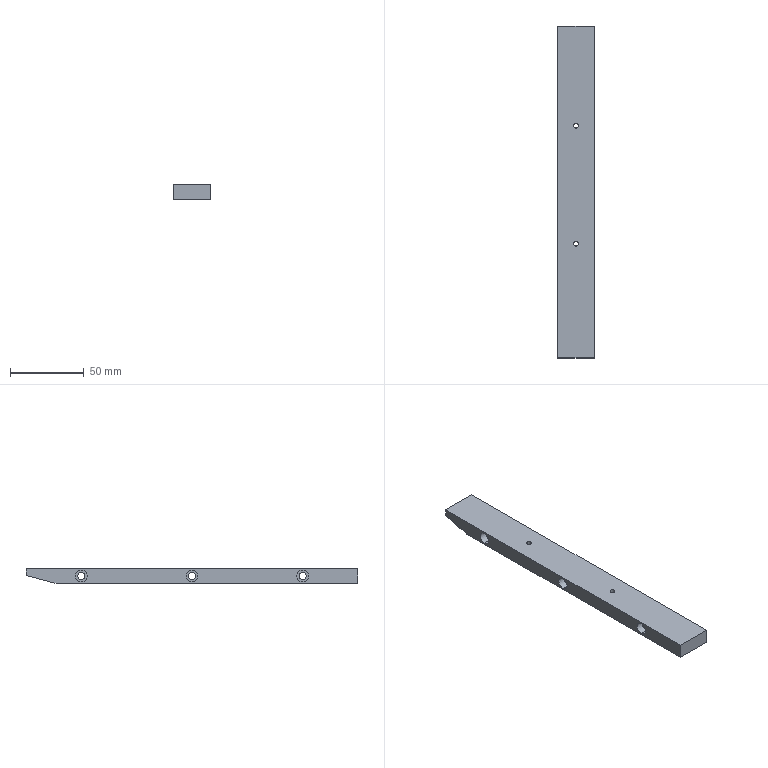Part | SolidWorks | features Chamfer 2, HoleWzd 2, Extrusion 1, Fillet 1 | 1 solid | 27 faces | box 25 x 225 x 10 mm | volume 52898 mm3 | cylinder 17 | plane 10 | commonest cylinder face diameters 4.8 x6 8 x6 3.3 x4 20 x1
STEP:
#1=CARTESIAN_POINT('',(-1.65,45.,-5.));
#2=VERTEX_POINT('',#1);
#3=CARTESIAN_POINT('',(1.65,45.,-5.));
#4=VERTEX_POINT('',#3);
#5=CARTESIAN_POINT('',(0.,45.,-5.));
#6=DIRECTION('',(0.,0.,1.));
#7=DIRECTION('',(1.,0.,0.));
#8=AXIS2_PLACEMENT_3D('',#5,#6,#7);
#9=CIRCLE('',#8,1.65);
#10=EDGE_CURVE('',#2,#4,#9,.T.);
#11=ORIENTED_EDGE('',*,*,#10,.F.);
#12=CARTESIAN_POINT('',(-1.65,45.,5.));
#13=VERTEX_POINT('',#12);
#14=CARTESIAN_POINT('',(-1.65,45.,5.));
#15=DIRECTION('',(0.,0.,1.));
#16=VECTOR('',#15,1000.);
#17=LINE('',#14,#16);
#18=EDGE_CURVE('',#2,#13,#17,.T.);
#19=ORIENTED_EDGE('',*,*,#18,.T.);
#20=CARTESIAN_POINT('',(1.65,45.,5.));
#21=VERTEX_POINT('',#20);
#22=CARTESIAN_POINT('',(0.,45.,5.));
#23=DIRECTION('',(0.,0.,1.));
#24=DIRECTION('',(1.,0.,0.));
#25=AXIS2_PLACEMENT_3D('',#22,#23,#24);
#26=CIRCLE('',#25,1.65);
#27=EDGE_CURVE('',#13,#21,#26,.T.);
#28=ORIENTED_EDGE('',*,*,#27,.T.);
#29=CARTESIAN_POINT('',(1.65,45.,5.));
#30=DIRECTION('',(0.,0.,1.));
#31=VECTOR('',#30,1000.);
#32=LINE('',#29,#31);
#33=EDGE_CURVE('',#4,#21,#32,.T.);
#34=ORIENTED_EDGE('',*,*,#33,.F.);
#35=EDGE_LOOP('',(#11,#19,#28,#34));
#36=FACE_OUTER_BOUND('',#35,.T.);
#37=CARTESIAN_POINT('',(0.,45.,5.));
#38=DIRECTION('',(0.,0.,1.));
#39=DIRECTION('',(1.,0.,0.));
#40=AXIS2_PLACEMENT_3D('',#37,#38,#39);
#41=CYLINDRICAL_SURFACE('',#40,1.65);
#42=ADVANCED_FACE('',(#36),#41,.F.);
#43=CARTESIAN_POINT('',(-1.65,-35.,-5.));
#44=VERTEX_POINT('',#43);
#45=CARTESIAN_POINT('',(1.65,-35.,-5.));
#46=VERTEX_POINT('',#45);
#47=CARTESIAN_POINT('',(0.,-35.,-5.));
#48=DIRECTION('',(0.,0.,1.));
#49=DIRECTION('',(1.,0.,0.));
#50=AXIS2_PLACEMENT_3D('',#47,#48,#49);
#51=CIRCLE('',#50,1.65);
#52=EDGE_CURVE('',#44,#46,#51,.T.);
#53=ORIENTED_EDGE('',*,*,#52,.F.);
#54=CARTESIAN_POINT('',(-1.65,-35.,5.));
#55=VERTEX_POINT('',#54);
#56=CARTESIAN_POINT('',(-1.65,-35.,5.));
#57=DIRECTION('',(0.,0.,1.));
#58=VECTOR('',#57,1000.);
#59=LINE('',#56,#58);
#60=EDGE_CURVE('',#44,#55,#59,.T.);
#61=ORIENTED_EDGE('',*,*,#60,.T.);
#62=CARTESIAN_POINT('',(1.65,-35.,5.));
#63=VERTEX_POINT('',#62);
#64=CARTESIAN_POINT('',(0.,-35.,5.));
#65=DIRECTION('',(0.,0.,1.));
#66=DIRECTION('',(1.,0.,0.));
#67=AXIS2_PLACEMENT_3D('',#64,#65,#66);
#68=CIRCLE('',#67,1.65);
#69=EDGE_CURVE('',#55,#63,#68,.T.);
#70=ORIENTED_EDGE('',*,*,#69,.T.);
#71=CARTESIAN_POINT('',(1.65,-35.,5.));
#72=DIRECTION('',(0.,0.,1.));
#73=VECTOR('',#72,1000.);
#74=LINE('',#71,#73);
#75=EDGE_CURVE('',#46,#63,#74,.T.);
#76=ORIENTED_EDGE('',*,*,#75,.F.);
#77=EDGE_LOOP('',(#53,#61,#70,#76));
#78=FACE_OUTER_BOUND('',#77,.T.);
#79=CARTESIAN_POINT('',(0.,-35.,5.));
#80=DIRECTION('',(0.,0.,1.));
#81=DIRECTION('',(1.,0.,0.));
#82=AXIS2_PLACEMENT_3D('',#79,#80,#81);
#83=CYLINDRICAL_SURFACE('',#82,1.65);
#84=ADVANCED_FACE('',(#78),#83,.F.);
#85=CARTESIAN_POINT('',(-7.5,75.,-4.));
#86=VERTEX_POINT('',#85);
#87=CARTESIAN_POINT('',(-7.5,75.,4.));
#88=VERTEX_POINT('',#87);
#89=CARTESIAN_POINT('',(-7.5,75.,0.));
#90=DIRECTION('',(-1.,0.,0.));
#91=DIRECTION('',(0.,0.,1.));
#92=AXIS2_PLACEMENT_3D('',#89,#90,#91);
#93=CIRCLE('',#92,4.);
#94=EDGE_CURVE('',#86,#88,#93,.T.);
#95=ORIENTED_EDGE('',*,*,#94,.F.);
#96=CARTESIAN_POINT('',(-12.5,75.,-4.));
#97=VERTEX_POINT('',#96);
#98=CARTESIAN_POINT('',(-12.5,75.,-4.));
#99=DIRECTION('',(-1.,0.,0.));
#100=VECTOR('',#99,1000.);
#101=LINE('',#98,#100);
#102=EDGE_CURVE('',#86,#97,#101,.T.);
#103=ORIENTED_EDGE('',*,*,#102,.T.);
#104=CARTESIAN_POINT('',(-12.5,75.,4.));
#105=VERTEX_POINT('',#104);
#106=CARTESIAN_POINT('',(-12.5,75.,0.));
#107=DIRECTION('',(-1.,0.,0.));
#108=DIRECTION('',(0.,0.,1.));
#109=AXIS2_PLACEMENT_3D('',#106,#107,#108);
#110=CIRCLE('',#109,4.);
#111=EDGE_CURVE('',#97,#105,#110,.T.);
#112=ORIENTED_EDGE('',*,*,#111,.T.);
#113=CARTESIAN_POINT('',(-12.5,75.,4.));
#114=DIRECTION('',(-1.,0.,0.));
#115=VECTOR('',#114,1000.);
#116=LINE('',#113,#115);
#117=EDGE_CURVE('',#88,#105,#116,.T.);
#118=ORIENTED_EDGE('',*,*,#117,.F.);
#119=EDGE_LOOP('',(#95,#103,#112,#118));
#120=FACE_OUTER_BOUND('',#119,.T.);
#121=CARTESIAN_POINT('',(-12.5,75.,0.));
#122=DIRECTION('',(-1.,0.,0.));
#123=DIRECTION('',(0.,0.,1.));
#124=AXIS2_PLACEMENT_3D('',#121,#122,#123);
#125=CYLINDRICAL_SURFACE('',#124,4.);
#126=ADVANCED_FACE('',(#120),#125,.F.);
#127=CARTESIAN_POINT('',(12.5,75.,-2.4));
#128=VERTEX_POINT('',#127);
#129=CARTESIAN_POINT('',(12.5,75.,2.4));
#130=VERTEX_POINT('',#129);
#131=CARTESIAN_POINT('',(12.5,75.,0.));
#132=DIRECTION('',(-1.,0.,0.));
#133=DIRECTION('',(0.,0.,1.));
#134=AXIS2_PLACEMENT_3D('',#131,#132,#133);
#135=CIRCLE('',#134,2.4);
#136=EDGE_CURVE('',#128,#130,#135,.T.);
#137=ORIENTED_EDGE('',*,*,#136,.F.);
#138=CARTESIAN_POINT('',(-7.5,75.,-2.4));
#139=VERTEX_POINT('',#138);
#140=CARTESIAN_POINT('',(-12.5,75.,-2.4));
#141=DIRECTION('',(-1.,0.,0.));
#142=VECTOR('',#141,1000.);
#143=LINE('',#140,#142);
#144=EDGE_CURVE('',#128,#139,#143,.T.);
#145=ORIENTED_EDGE('',*,*,#144,.T.);
#146=CARTESIAN_POINT('',(-7.5,75.,2.4));
#147=VERTEX_POINT('',#146);
#148=CARTESIAN_POINT('',(-7.5,75.,0.));
#149=DIRECTION('',(-1.,0.,0.));
#150=DIRECTION('',(0.,0.,1.));
#151=AXIS2_PLACEMENT_3D('',#148,#149,#150);
#152=CIRCLE('',#151,2.4);
#153=EDGE_CURVE('',#139,#147,#152,.T.);
#154=ORIENTED_EDGE('',*,*,#153,.T.);
#155=CARTESIAN_POINT('',(-12.5,75.,2.4));
#156=DIRECTION('',(-1.,0.,0.));
#157=VECTOR('',#156,1000.);
#158=LINE('',#155,#157);
#159=EDGE_CURVE('',#130,#147,#158,.T.);
#160=ORIENTED_EDGE('',*,*,#159,.F.);
#161=EDGE_LOOP('',(#137,#145,#154,#160));
#162=FACE_OUTER_BOUND('',#161,.T.);
#163=CARTESIAN_POINT('',(-12.5,75.,0.));
#164=DIRECTION('',(-1.,0.,0.));
#165=DIRECTION('',(0.,0.,1.));
#166=AXIS2_PLACEMENT_3D('',#163,#164,#165);
#167=CYLINDRICAL_SURFACE('',#166,2.4);
#168=ADVANCED_FACE('',(#162),#167,.F.);
#169=CARTESIAN_POINT('',(-7.5,0.,-4.));
#170=VERTEX_POINT('',#169);
#171=CARTESIAN_POINT('',(-7.5,0.,4.));
#172=VERTEX_POINT('',#171);
#173=CARTESIAN_POINT('',(-7.5,0.,0.));
#174=DIRECTION('',(-1.,0.,0.));
#175=DIRECTION('',(0.,0.,1.));
#176=AXIS2_PLACEMENT_3D('',#173,#174,#175);
#177=CIRCLE('',#176,4.);
#178=EDGE_CURVE('',#170,#172,#177,.T.);
#179=ORIENTED_EDGE('',*,*,#178,.F.);
#180=CARTESIAN_POINT('',(-12.5,0.,-4.));
#181=VERTEX_POINT('',#180);
#182=CARTESIAN_POINT('',(-12.5,0.,-4.));
#183=DIRECTION('',(-1.,0.,0.));
#184=VECTOR('',#183,1000.);
#185=LINE('',#182,#184);
#186=EDGE_CURVE('',#170,#181,#185,.T.);
#187=ORIENTED_EDGE('',*,*,#186,.T.);
#188=CARTESIAN_POINT('',(-12.5,0.,4.));
#189=VERTEX_POINT('',#188);
#190=CARTESIAN_POINT('',(-12.5,0.,0.));
#191=DIRECTION('',(-1.,0.,0.));
#192=DIRECTION('',(0.,0.,1.));
#193=AXIS2_PLACEMENT_3D('',#190,#191,#192);
#194=CIRCLE('',#193,4.);
#195=EDGE_CURVE('',#181,#189,#194,.T.);
#196=ORIENTED_EDGE('',*,*,#195,.T.);
#197=CARTESIAN_POINT('',(-12.5,0.,4.));
#198=DIRECTION('',(-1.,0.,0.));
#199=VECTOR('',#198,1000.);
#200=LINE('',#197,#199);
#201=EDGE_CURVE('',#172,#189,#200,.T.);
#202=ORIENTED_EDGE('',*,*,#201,.F.);
#203=EDGE_LOOP('',(#179,#187,#196,#202));
#204=FACE_OUTER_BOUND('',#203,.T.);
#205=CARTESIAN_POINT('',(-12.5,0.,0.));
#206=DIRECTION('',(-1.,0.,0.));
#207=DIRECTION('',(0.,0.,1.));
#208=AXIS2_PLACEMENT_3D('',#205,#206,#207);
#209=CYLINDRICAL_SURFACE('',#208,4.);
#210=ADVANCED_FACE('',(#204),#209,.F.);
#211=CARTESIAN_POINT('',(12.5,0.,-2.4));
#212=VERTEX_POINT('',#211);
#213=CARTESIAN_POINT('',(12.5,0.,2.4));
#214=VERTEX_POINT('',#213);
#215=CARTESIAN_POINT('',(12.5,0.,0.));
#216=DIRECTION('',(-1.,0.,0.));
#217=DIRECTION('',(0.,0.,1.));
#218=AXIS2_PLACEMENT_3D('',#215,#216,#217);
#219=CIRCLE('',#218,2.4);
#220=EDGE_CURVE('',#212,#214,#219,.T.);
#221=ORIENTED_EDGE('',*,*,#220,.F.);
#222=CARTESIAN_POINT('',(-7.5,0.,-2.4));
#223=VERTEX_POINT('',#222);
#224=CARTESIAN_POINT('',(-12.5,0.,-2.4));
#225=DIRECTION('',(-1.,0.,0.));
#226=VECTOR('',#225,1000.);
#227=LINE('',#224,#226);
#228=EDGE_CURVE('',#212,#223,#227,.T.);
#229=ORIENTED_EDGE('',*,*,#228,.T.);
#230=CARTESIAN_POINT('',(-7.5,0.,2.4));
#231=VERTEX_POINT('',#230);
#232=CARTESIAN_POINT('',(-7.5,0.,0.));
#233=DIRECTION('',(-1.,0.,0.));
#234=DIRECTION('',(0.,0.,1.));
#235=AXIS2_PLACEMENT_3D('',#232,#233,#234);
#236=CIRCLE('',#235,2.4);
#237=EDGE_CURVE('',#223,#231,#236,.T.);
#238=ORIENTED_EDGE('',*,*,#237,.T.);
#239=CARTESIAN_POINT('',(-12.5,0.,2.4));
#240=DIRECTION('',(-1.,0.,0.));
#241=VECTOR('',#240,1000.);
#242=LINE('',#239,#241);
#243=EDGE_CURVE('',#214,#231,#242,.T.);
#244=ORIENTED_EDGE('',*,*,#243,.F.);
#245=EDGE_LOOP('',(#221,#229,#238,#244));
#246=FACE_OUTER_BOUND('',#245,.T.);
#247=CARTESIAN_POINT('',(-12.5,0.,0.));
#248=DIRECTION('',(-1.,0.,0.));
#249=DIRECTION('',(0.,0.,1.));
#250=AXIS2_PLACEMENT_3D('',#247,#248,#249);
#251=CYLINDRICAL_SURFACE('',#250,2.4);
#252=ADVANCED_FACE('',(#246),#251,.F.);
#253=CARTESIAN_POINT('',(-7.5,-75.,-4.));
#254=VERTEX_POINT('',#253);
#255=CARTESIAN_POINT('',(-7.5,-75.,4.));
#256=VERTEX_POINT('',#255);
#257=CARTESIAN_POINT('',(-7.5,-75.,0.));
#258=DIRECTION('',(-1.,0.,0.));
#259=DIRECTION('',(0.,0.,1.));
#260=AXIS2_PLACEMENT_3D('',#257,#258,#259);
#261=CIRCLE('',#260,4.);
#262=EDGE_CURVE('',#254,#256,#261,.T.);
#263=ORIENTED_EDGE('',*,*,#262,.F.);
#264=CARTESIAN_POINT('',(-12.5,-75.,-4.));
#265=VERTEX_POINT('',#264);
#266=CARTESIAN_POINT('',(-12.5,-75.,-4.));
#267=DIRECTION('',(-1.,0.,0.));
#268=VECTOR('',#267,1000.);
#269=LINE('',#266,#268);
#270=EDGE_CURVE('',#254,#265,#269,.T.);
#271=ORIENTED_EDGE('',*,*,#270,.T.);
#272=CARTESIAN_POINT('',(-12.5,-75.,4.));
#273=VERTEX_POINT('',#272);
#274=CARTESIAN_POINT('',(-12.5,-75.,0.));
#275=DIRECTION('',(-1.,0.,0.));
#276=DIRECTION('',(0.,0.,1.));
#277=AXIS2_PLACEMENT_3D('',#274,#275,#276);
#278=CIRCLE('',#277,4.);
#279=EDGE_CURVE('',#265,#273,#278,.T.);
#280=ORIENTED_EDGE('',*,*,#279,.T.);
#281=CARTESIAN_POINT('',(-12.5,-75.,4.));
#282=DIRECTION('',(-1.,0.,0.));
#283=VECTOR('',#282,1000.);
#284=LINE('',#281,#283);
#285=EDGE_CURVE('',#256,#273,#284,.T.);
#286=ORIENTED_EDGE('',*,*,#285,.F.);
#287=EDGE_LOOP('',(#263,#271,#280,#286));
#288=FACE_OUTER_BOUND('',#287,.T.);
#289=CARTESIAN_POINT('',(-12.5,-75.,0.));
#290=DIRECTION('',(-1.,0.,0.));
#291=DIRECTION('',(0.,0.,1.));
#292=AXIS2_PLACEMENT_3D('',#289,#290,#291);
#293=CYLINDRICAL_SURFACE('',#292,4.);
#294=ADVANCED_FACE('',(#288),#293,.F.);
#295=CARTESIAN_POINT('',(12.5,-75.,-2.4));
#296=VERTEX_POINT('',#295);
#297=CARTESIAN_POINT('',(12.5,-75.,2.4));
#298=VERTEX_POINT('',#297);
#299=CARTESIAN_POINT('',(12.5,-75.,0.));
#300=DIRECTION('',(-1.,0.,0.));
#301=DIRECTION('',(0.,0.,1.));
#302=AXIS2_PLACEMENT_3D('',#299,#300,#301);
#303=CIRCLE('',#302,2.4);
#304=EDGE_CURVE('',#296,#298,#303,.T.);
#305=ORIENTED_EDGE('',*,*,#304,.F.);
#306=CARTESIAN_POINT('',(-7.5,-75.,-2.4));
#307=VERTEX_POINT('',#306);
#308=CARTESIAN_POINT('',(-12.5,-75.,-2.4));
#309=DIRECTION('',(-1.,0.,0.));
#310=VECTOR('',#309,1000.);
#311=LINE('',#308,#310);
#312=EDGE_CURVE('',#296,#307,#311,.T.);
#313=ORIENTED_EDGE('',*,*,#312,.T.);
#314=CARTESIAN_POINT('',(-7.5,-75.,2.4));
#315=VERTEX_POINT('',#314);
#316=CARTESIAN_POINT('',(-7.5,-75.,0.));
#317=DIRECTION('',(-1.,0.,0.));
#318=DIRECTION('',(0.,0.,1.));
#319=AXIS2_PLACEMENT_3D('',#316,#317,#318);
#320=CIRCLE('',#319,2.4);
#321=EDGE_CURVE('',#307,#315,#320,.T.);
#322=ORIENTED_EDGE('',*,*,#321,.T.);
#323=CARTESIAN_POINT('',(-12.5,-75.,2.4));
#324=DIRECTION('',(-1.,0.,0.));
#325=VECTOR('',#324,1000.);
#326=LINE('',#323,#325);
#327=EDGE_CURVE('',#298,#315,#326,.T.);
#328=ORIENTED_EDGE('',*,*,#327,.F.);
#329=EDGE_LOOP('',(#305,#313,#322,#328));
#330=FACE_OUTER_BOUND('',#329,.T.);
#331=CARTESIAN_POINT('',(-12.5,-75.,0.));
#332=DIRECTION('',(-1.,0.,0.));
#333=DIRECTION('',(0.,0.,1.));
#334=AXIS2_PLACEMENT_3D('',#331,#332,#333);
#335=CYLINDRICAL_SURFACE('',#334,2.4);
#336=ADVANCED_FACE('',(#330),#335,.F.);
#337=CARTESIAN_POINT('',(0.,45.,-5.));
#338=DIRECTION('',(0.,0.,1.));
#339=DIRECTION('',(1.,0.,0.));
#340=AXIS2_PLACEMENT_3D('',#337,#338,#339);
#341=CIRCLE('',#340,1.65);
#342=EDGE_CURVE('',#4,#2,#341,.T.);
#343=ORIENTED_EDGE('',*,*,#342,.T.);
#344=ORIENTED_EDGE('',*,*,#10,.T.);
#345=EDGE_LOOP('',(#343,#344));
#346=FACE_BOUND('',#345,.T.);
#347=CARTESIAN_POINT('',(0.,-35.,-5.));
#348=DIRECTION('',(0.,0.,1.));
#349=DIRECTION('',(1.,0.,0.));
#350=AXIS2_PLACEMENT_3D('',#347,#348,#349);
#351=CIRCLE('',#350,1.65);
#352=EDGE_CURVE('',#46,#44,#351,.T.);
#353=ORIENTED_EDGE('',*,*,#352,.T.);
#354=ORIENTED_EDGE('',*,*,#52,.T.);
#355=EDGE_LOOP('',(#353,#354));
#356=FACE_BOUND('',#355,.T.);
#357=CARTESIAN_POINT('',(-12.5,-112.5,-5.));
#358=VERTEX_POINT('',#357);
#359=CARTESIAN_POINT('',(-12.5,91.183,-5.));
#360=VERTEX_POINT('',#359);
#361=CARTESIAN_POINT('',(-12.5,112.5,-5.));
#362=DIRECTION('',(0.,1.,0.));
#363=VECTOR('',#362,1000.);
#364=LINE('',#361,#363);
#365=EDGE_CURVE('',#358,#360,#364,.T.);
#366=ORIENTED_EDGE('',*,*,#365,.T.);
#367=CARTESIAN_POINT('',(12.5,91.183,-5.));
#368=VERTEX_POINT('',#367);
#369=CARTESIAN_POINT('',(12.5,91.183,-5.));
#370=DIRECTION('',(1.,0.,0.));
#371=VECTOR('',#370,1000.);
#372=LINE('',#369,#371);
#373=EDGE_CURVE('',#360,#368,#372,.T.);
#374=ORIENTED_EDGE('',*,*,#373,.T.);
#375=CARTESIAN_POINT('',(12.5,-112.5,-5.));
#376=VERTEX_POINT('',#375);
#377=CARTESIAN_POINT('',(12.5,112.5,-5.));
#378=DIRECTION('',(0.,1.,0.));
#379=VECTOR('',#378,1000.);
#380=LINE('',#377,#379);
#381=EDGE_CURVE('',#376,#368,#380,.T.);
#382=ORIENTED_EDGE('',*,*,#381,.F.);
#383=CARTESIAN_POINT('',(12.5,-112.5,-5.));
#384=DIRECTION('',(-1.,0.,0.));
#385=VECTOR('',#384,1000.);
#386=LINE('',#383,#385);
#387=EDGE_CURVE('',#376,#358,#386,.T.);
#388=ORIENTED_EDGE('',*,*,#387,.T.);
#389=EDGE_LOOP('',(#366,#374,#382,#388));
#390=FACE_OUTER_BOUND('',#389,.T.);
#391=CARTESIAN_POINT('',(12.5,112.5,-5.));
#392=DIRECTION('',(0.,0.,1.));
#393=DIRECTION('',(0.,-1.,0.));
#394=AXIS2_PLACEMENT_3D('',#391,#392,#393);
#395=PLANE('',#394);
#396=ADVANCED_FACE('',(#346,#356,#390),#395,.F.);
#397=CARTESIAN_POINT('',(12.5,112.5,0.359));
#398=VERTEX_POINT('',#397);
#399=CARTESIAN_POINT('',(12.5,112.5,5.));
#400=VERTEX_POINT('',#399);
#401=CARTESIAN_POINT('',(12.5,112.5,5.));
#402=DIRECTION('',(0.,0.,1.));
#403=VECTOR('',#402,1000.);
#404=LINE('',#401,#403);
#405=EDGE_CURVE('',#398,#400,#404,.T.);
#406=ORIENTED_EDGE('',*,*,#405,.F.);
#407=CARTESIAN_POINT('',(-12.5,112.5,0.359));
#408=VERTEX_POINT('',#407);
#409=CARTESIAN_POINT('',(12.5,112.5,0.359));
#410=DIRECTION('',(-1.,0.,0.));
#411=VECTOR('',#410,1000.);
#412=LINE('',#409,#411);
#413=EDGE_CURVE('',#398,#408,#412,.T.);
#414=ORIENTED_EDGE('',*,*,#413,.T.);
#415=CARTESIAN_POINT('',(-12.5,112.5,5.));
#416=VERTEX_POINT('',#415);
#417=CARTESIAN_POINT('',(-12.5,112.5,5.));
#418=DIRECTION('',(0.,0.,1.));
#419=VECTOR('',#418,1000.);
#420=LINE('',#417,#419);
#421=EDGE_CURVE('',#408,#416,#420,.T.);
#422=ORIENTED_EDGE('',*,*,#421,.T.);
#423=CARTESIAN_POINT('',(12.5,112.5,5.));
#424=DIRECTION('',(-1.,0.,0.));
#425=VECTOR('',#424,1000.);
#426=LINE('',#423,#425);
#427=EDGE_CURVE('',#400,#416,#426,.T.);
#428=ORIENTED_EDGE('',*,*,#427,.F.);
#429=EDGE_LOOP('',(#406,#414,#422,#428));
#430=FACE_OUTER_BOUND('',#429,.T.);
#431=CARTESIAN_POINT('',(12.5,112.5,5.));
#432=DIRECTION('',(0.,-1.,0.));
#433=DIRECTION('',(0.,0.,-1.));
#434=AXIS2_PLACEMENT_3D('',#431,#432,#433);
#435=PLANE('',#434);
#436=ADVANCED_FACE('',(#430),#435,.F.);
#437=CARTESIAN_POINT('',(0.,45.,5.));
#438=DIRECTION('',(0.,0.,1.));
#439=DIRECTION('',(1.,0.,0.));
#440=AXIS2_PLACEMENT_3D('',#437,#438,#439);
#441=CIRCLE('',#440,1.65);
#442=EDGE_CURVE('',#21,#13,#441,.T.);
#443=ORIENTED_EDGE('',*,*,#442,.F.);
#444=ORIENTED_EDGE('',*,*,#27,.F.);
#445=EDGE_LOOP('',(#443,#444));
#446=FACE_BOUND('',#445,.T.);
#447=CARTESIAN_POINT('',(0.,-35.,5.));
#448=DIRECTION('',(0.,0.,1.));
#449=DIRECTION('',(1.,0.,0.));
#450=AXIS2_PLACEMENT_3D('',#447,#448,#449);
#451=CIRCLE('',#450,1.65);
#452=EDGE_CURVE('',#63,#55,#451,.T.);
#453=ORIENTED_EDGE('',*,*,#452,.F.);
#454=ORIENTED_EDGE('',*,*,#69,.F.);
#455=EDGE_LOOP('',(#453,#454));
#456=FACE_BOUND('',#455,.T.);
#457=CARTESIAN_POINT('',(-12.5,-112.5,5.));
#458=VERTEX_POINT('',#457);
#459=CARTESIAN_POINT('',(-12.5,112.5,5.));
#460=DIRECTION('',(0.,-1.,0.));
#461=VECTOR('',#460,1000.);
#462=LINE('',#459,#461);
#463=EDGE_CURVE('',#416,#458,#462,.T.);
#464=ORIENTED_EDGE('',*,*,#463,.T.);
#465=CARTESIAN_POINT('',(12.5,-112.5,5.));
#466=VERTEX_POINT('',#465);
#467=CARTESIAN_POINT('',(12.5,-112.5,5.));
#468=DIRECTION('',(-1.,0.,0.));
#469=VECTOR('',#468,1000.);
#470=LINE('',#467,#469);
#471=EDGE_CURVE('',#466,#458,#470,.T.);
#472=ORIENTED_EDGE('',*,*,#471,.F.);
#473=CARTESIAN_POINT('',(12.5,112.5,5.));
#474=DIRECTION('',(0.,-1.,0.));
#475=VECTOR('',#474,1000.);
#476=LINE('',#473,#475);
#477=EDGE_CURVE('',#400,#466,#476,.T.);
#478=ORIENTED_EDGE('',*,*,#477,.F.);
#479=ORIENTED_EDGE('',*,*,#427,.T.);
#480=EDGE_LOOP('',(#464,#472,#478,#479));
#481=FACE_OUTER_BOUND('',#480,.T.);
#482=CARTESIAN_POINT('',(12.5,112.5,5.));
#483=DIRECTION('',(0.,0.,-1.));
#484=DIRECTION('',(0.,1.,0.));
#485=AXIS2_PLACEMENT_3D('',#482,#483,#484);
#486=PLANE('',#485);
#487=ADVANCED_FACE('',(#446,#456,#481),#486,.F.);
#488=CARTESIAN_POINT('',(-12.5,-112.5,5.));
#489=DIRECTION('',(0.,0.,-1.));
#490=VECTOR('',#489,1000.);
#491=LINE('',#488,#490);
#492=EDGE_CURVE('',#458,#358,#491,.T.);
#493=ORIENTED_EDGE('',*,*,#492,.T.);
#494=ORIENTED_EDGE('',*,*,#387,.F.);
#495=CARTESIAN_POINT('',(12.5,-112.5,5.));
#496=DIRECTION('',(0.,0.,-1.));
#497=VECTOR('',#496,1000.);
#498=LINE('',#495,#497);
#499=EDGE_CURVE('',#466,#376,#498,.T.);
#500=ORIENTED_EDGE('',*,*,#499,.F.);
#501=ORIENTED_EDGE('',*,*,#471,.T.);
#502=EDGE_LOOP('',(#493,#494,#500,#501));
#503=FACE_OUTER_BOUND('',#502,.T.);
#504=CARTESIAN_POINT('',(12.5,-112.5,5.));
#505=DIRECTION('',(0.,1.,0.));
#506=DIRECTION('',(0.,0.,1.));
#507=AXIS2_PLACEMENT_3D('',#504,#505,#506);
#508=PLANE('',#507);
#509=ADVANCED_FACE('',(#503),#508,.F.);
#510=CARTESIAN_POINT('',(12.5,75.,0.));
#511=DIRECTION('',(-1.,0.,0.));
#512=DIRECTION('',(0.,0.,1.));
#513=AXIS2_PLACEMENT_3D('',#510,#511,#512);
#514=CIRCLE('',#513,2.4);
#515=EDGE_CURVE('',#130,#128,#514,.T.);
#516=ORIENTED_EDGE('',*,*,#515,.T.);
#517=ORIENTED_EDGE('',*,*,#136,.T.);
#518=EDGE_LOOP('',(#516,#517));
#519=FACE_BOUND('',#518,.T.);
#520=CARTESIAN_POINT('',(12.5,0.,0.));
#521=DIRECTION('',(-1.,0.,0.));
#522=DIRECTION('',(0.,0.,1.));
#523=AXIS2_PLACEMENT_3D('',#520,#521,#522);
#524=CIRCLE('',#523,2.4);
#525=EDGE_CURVE('',#214,#212,#524,.T.);
#526=ORIENTED_EDGE('',*,*,#525,.T.);
#527=ORIENTED_EDGE('',*,*,#220,.T.);
#528=EDGE_LOOP('',(#526,#527));
#529=FACE_BOUND('',#528,.T.);
#530=CARTESIAN_POINT('',(12.5,-75.,0.));
#531=DIRECTION('',(-1.,0.,0.));
#532=DIRECTION('',(0.,0.,1.));
#533=AXIS2_PLACEMENT_3D('',#530,#531,#532);
#534=CIRCLE('',#533,2.4);
#535=EDGE_CURVE('',#298,#296,#534,.T.);
#536=ORIENTED_EDGE('',*,*,#535,.T.);
#537=ORIENTED_EDGE('',*,*,#304,.T.);
#538=EDGE_LOOP('',(#536,#537));
#539=FACE_BOUND('',#538,.T.);
#540=ORIENTED_EDGE('',*,*,#381,.T.);
#541=CARTESIAN_POINT('',(12.5,93.772,-4.659));
#542=VERTEX_POINT('',#541);
#543=CARTESIAN_POINT('',(12.5,91.183,5.));
#544=DIRECTION('',(1.,0.,0.));
#545=DIRECTION('',(0.,0.,-1.));
#546=AXIS2_PLACEMENT_3D('',#543,#544,#545);
#547=CIRCLE('',#546,10.);
#548=EDGE_CURVE('',#368,#542,#547,.T.);
#549=ORIENTED_EDGE('',*,*,#548,.T.);
#550=CARTESIAN_POINT('',(12.5,7.446,-27.79));
#551=DIRECTION('',(0.,0.9659,0.2588));
#552=VECTOR('',#551,1000.);
#553=LINE('',#550,#552);
#554=EDGE_CURVE('',#542,#398,#553,.T.);
#555=ORIENTED_EDGE('',*,*,#554,.T.);
#556=ORIENTED_EDGE('',*,*,#405,.T.);
#557=ORIENTED_EDGE('',*,*,#477,.T.);
#558=ORIENTED_EDGE('',*,*,#499,.T.);
#559=EDGE_LOOP('',(#540,#549,#555,#556,#557,#558));
#560=FACE_OUTER_BOUND('',#559,.T.);
#561=CARTESIAN_POINT('',(12.5,0.,0.));
#562=DIRECTION('',(1.,0.,0.));
#563=DIRECTION('',(0.,0.,-1.));
#564=AXIS2_PLACEMENT_3D('',#561,#562,#563);
#565=PLANE('',#564);
#566=ADVANCED_FACE('',(#519,#529,#539,#560),#565,.T.);
#567=CARTESIAN_POINT('',(-12.5,75.,0.));
#568=DIRECTION('',(-1.,0.,0.));
#569=DIRECTION('',(0.,0.,1.));
#570=AXIS2_PLACEMENT_3D('',#567,#568,#569);
#571=CIRCLE('',#570,4.);
#572=EDGE_CURVE('',#105,#97,#571,.T.);
#573=ORIENTED_EDGE('',*,*,#572,.F.);
#574=ORIENTED_EDGE('',*,*,#111,.F.);
#575=EDGE_LOOP('',(#573,#574));
#576=FACE_BOUND('',#575,.T.);
#577=CARTESIAN_POINT('',(-12.5,0.,0.));
#578=DIRECTION('',(-1.,0.,0.));
#579=DIRECTION('',(0.,0.,1.));
#580=AXIS2_PLACEMENT_3D('',#577,#578,#579);
#581=CIRCLE('',#580,4.);
#582=EDGE_CURVE('',#189,#181,#581,.T.);
#583=ORIENTED_EDGE('',*,*,#582,.F.);
#584=ORIENTED_EDGE('',*,*,#195,.F.);
#585=EDGE_LOOP('',(#583,#584));
#586=FACE_BOUND('',#585,.T.);
#587=CARTESIAN_POINT('',(-12.5,-75.,0.));
#588=DIRECTION('',(-1.,0.,0.));
#589=DIRECTION('',(0.,0.,1.));
#590=AXIS2_PLACEMENT_3D('',#587,#588,#589);
#591=CIRCLE('',#590,4.);
#592=EDGE_CURVE('',#273,#265,#591,.T.);
#593=ORIENTED_EDGE('',*,*,#592,.F.);
#594=ORIENTED_EDGE('',*,*,#279,.F.);
#595=EDGE_LOOP('',(#593,#594));
#596=FACE_BOUND('',#595,.T.);
#597=CARTESIAN_POINT('',(-12.5,93.772,-4.659));
#598=VERTEX_POINT('',#597);
#599=CARTESIAN_POINT('',(-12.5,112.5,0.359));
#600=DIRECTION('',(0.,-0.9659,-0.2588));
#601=VECTOR('',#600,1000.);
#602=LINE('',#599,#601);
#603=EDGE_CURVE('',#408,#598,#602,.T.);
#604=ORIENTED_EDGE('',*,*,#603,.T.);
#605=CARTESIAN_POINT('',(-12.5,91.183,5.));
#606=DIRECTION('',(-1.,0.,0.));
#607=DIRECTION('',(0.,0.,-1.));
#608=AXIS2_PLACEMENT_3D('',#605,#606,#607);
#609=CIRCLE('',#608,10.);
#610=EDGE_CURVE('',#598,#360,#609,.T.);
#611=ORIENTED_EDGE('',*,*,#610,.T.);
#612=ORIENTED_EDGE('',*,*,#365,.F.);
#613=ORIENTED_EDGE('',*,*,#492,.F.);
#614=ORIENTED_EDGE('',*,*,#463,.F.);
#615=ORIENTED_EDGE('',*,*,#421,.F.);
#616=EDGE_LOOP('',(#604,#611,#612,#613,#614,#615));
#617=FACE_OUTER_BOUND('',#616,.T.);
#618=CARTESIAN_POINT('',(-12.5,0.,0.));
#619=DIRECTION('',(1.,0.,0.));
#620=DIRECTION('',(0.,0.,-1.));
#621=AXIS2_PLACEMENT_3D('',#618,#619,#620);
#622=PLANE('',#621);
#623=ADVANCED_FACE('',(#576,#586,#596,#617),#622,.F.);
#624=ORIENTED_EDGE('',*,*,#554,.F.);
#625=CARTESIAN_POINT('',(-12.5,93.772,-4.659));
#626=DIRECTION('',(-1.,0.,0.));
#627=VECTOR('',#626,1000.);
#628=LINE('',#625,#627);
#629=EDGE_CURVE('',#542,#598,#628,.T.);
#630=ORIENTED_EDGE('',*,*,#629,.T.);
#631=ORIENTED_EDGE('',*,*,#603,.F.);
#632=ORIENTED_EDGE('',*,*,#413,.F.);
#633=EDGE_LOOP('',(#624,#630,#631,#632));
#634=FACE_OUTER_BOUND('',#633,.T.);
#635=CARTESIAN_POINT('',(12.5,112.5,0.359));
#636=DIRECTION('',(0.,-0.2588,0.9659));
#637=DIRECTION('',(-1.,0.,0.));
#638=AXIS2_PLACEMENT_3D('',#635,#636,#637);
#639=PLANE('',#638);
#640=ADVANCED_FACE('',(#634),#639,.F.);
#641=ORIENTED_EDGE('',*,*,#312,.F.);
#642=ORIENTED_EDGE('',*,*,#535,.F.);
#643=ORIENTED_EDGE('',*,*,#327,.T.);
#644=CARTESIAN_POINT('',(-7.5,-75.,0.));
#645=DIRECTION('',(-1.,0.,0.));
#646=DIRECTION('',(0.,0.,1.));
#647=AXIS2_PLACEMENT_3D('',#644,#645,#646);
#648=CIRCLE('',#647,2.4);
#649=EDGE_CURVE('',#315,#307,#648,.T.);
#650=ORIENTED_EDGE('',*,*,#649,.T.);
#651=EDGE_LOOP('',(#641,#642,#643,#650));
#652=FACE_OUTER_BOUND('',#651,.T.);
#653=CARTESIAN_POINT('',(-12.5,-75.,0.));
#654=DIRECTION('',(-1.,0.,0.));
#655=DIRECTION('',(0.,0.,1.));
#656=AXIS2_PLACEMENT_3D('',#653,#654,#655);
#657=CYLINDRICAL_SURFACE('',#656,2.4);
#658=ADVANCED_FACE('',(#652),#657,.F.);
#659=ORIENTED_EDGE('',*,*,#649,.F.);
#660=ORIENTED_EDGE('',*,*,#321,.F.);
#661=EDGE_LOOP('',(#659,#660));
#662=FACE_BOUND('',#661,.T.);
#663=CARTESIAN_POINT('',(-7.5,-75.,0.));
#664=DIRECTION('',(-1.,0.,0.));
#665=DIRECTION('',(0.,0.,1.));
#666=AXIS2_PLACEMENT_3D('',#663,#664,#665);
#667=CIRCLE('',#666,4.);
#668=EDGE_CURVE('',#256,#254,#667,.T.);
#669=ORIENTED_EDGE('',*,*,#668,.T.);
#670=ORIENTED_EDGE('',*,*,#262,.T.);
#671=EDGE_LOOP('',(#669,#670));
#672=FACE_OUTER_BOUND('',#671,.T.);
#673=CARTESIAN_POINT('',(-7.5,-72.6,0.));
#674=DIRECTION('',(1.,0.,0.));
#675=DIRECTION('',(0.,0.,-1.));
#676=AXIS2_PLACEMENT_3D('',#673,#674,#675);
#677=PLANE('',#676);
#678=ADVANCED_FACE('',(#662,#672),#677,.F.);
#679=ORIENTED_EDGE('',*,*,#270,.F.);
#680=ORIENTED_EDGE('',*,*,#668,.F.);
#681=ORIENTED_EDGE('',*,*,#285,.T.);
#682=ORIENTED_EDGE('',*,*,#592,.T.);
#683=EDGE_LOOP('',(#679,#680,#681,#682));
#684=FACE_OUTER_BOUND('',#683,.T.);
#685=CARTESIAN_POINT('',(-12.5,-75.,0.));
#686=DIRECTION('',(-1.,0.,0.));
#687=DIRECTION('',(0.,0.,1.));
#688=AXIS2_PLACEMENT_3D('',#685,#686,#687);
#689=CYLINDRICAL_SURFACE('',#688,4.);
#690=ADVANCED_FACE('',(#684),#689,.F.);
#691=ORIENTED_EDGE('',*,*,#228,.F.);
#692=ORIENTED_EDGE('',*,*,#525,.F.);
#693=ORIENTED_EDGE('',*,*,#243,.T.);
#694=CARTESIAN_POINT('',(-7.5,0.,0.));
#695=DIRECTION('',(-1.,0.,0.));
#696=DIRECTION('',(0.,0.,1.));
#697=AXIS2_PLACEMENT_3D('',#694,#695,#696);
#698=CIRCLE('',#697,2.4);
#699=EDGE_CURVE('',#231,#223,#698,.T.);
#700=ORIENTED_EDGE('',*,*,#699,.T.);
#701=EDGE_LOOP('',(#691,#692,#693,#700));
#702=FACE_OUTER_BOUND('',#701,.T.);
#703=CARTESIAN_POINT('',(-12.5,0.,0.));
#704=DIRECTION('',(-1.,0.,0.));
#705=DIRECTION('',(0.,0.,1.));
#706=AXIS2_PLACEMENT_3D('',#703,#704,#705);
#707=CYLINDRICAL_SURFACE('',#706,2.4);
#708=ADVANCED_FACE('',(#702),#707,.F.);
#709=ORIENTED_EDGE('',*,*,#699,.F.);
#710=ORIENTED_EDGE('',*,*,#237,.F.);
#711=EDGE_LOOP('',(#709,#710));
#712=FACE_BOUND('',#711,.T.);
#713=CARTESIAN_POINT('',(-7.5,0.,0.));
#714=DIRECTION('',(-1.,0.,0.));
#715=DIRECTION('',(0.,0.,1.));
#716=AXIS2_PLACEMENT_3D('',#713,#714,#715);
#717=CIRCLE('',#716,4.);
#718=EDGE_CURVE('',#172,#170,#717,.T.);
#719=ORIENTED_EDGE('',*,*,#718,.T.);
#720=ORIENTED_EDGE('',*,*,#178,.T.);
#721=EDGE_LOOP('',(#719,#720));
#722=FACE_OUTER_BOUND('',#721,.T.);
#723=CARTESIAN_POINT('',(-7.5,2.4,0.));
#724=DIRECTION('',(1.,0.,0.));
#725=DIRECTION('',(0.,0.,-1.));
#726=AXIS2_PLACEMENT_3D('',#723,#724,#725);
#727=PLANE('',#726);
#728=ADVANCED_FACE('',(#712,#722),#727,.F.);
#729=ORIENTED_EDGE('',*,*,#186,.F.);
#730=ORIENTED_EDGE('',*,*,#718,.F.);
#731=ORIENTED_EDGE('',*,*,#201,.T.);
#732=ORIENTED_EDGE('',*,*,#582,.T.);
#733=EDGE_LOOP('',(#729,#730,#731,#732));
#734=FACE_OUTER_BOUND('',#733,.T.);
#735=CARTESIAN_POINT('',(-12.5,0.,0.));
#736=DIRECTION('',(-1.,0.,0.));
#737=DIRECTION('',(0.,0.,1.));
#738=AXIS2_PLACEMENT_3D('',#735,#736,#737);
#739=CYLINDRICAL_SURFACE('',#738,4.);
#740=ADVANCED_FACE('',(#734),#739,.F.);
#741=ORIENTED_EDGE('',*,*,#144,.F.);
#742=ORIENTED_EDGE('',*,*,#515,.F.);
#743=ORIENTED_EDGE('',*,*,#159,.T.);
#744=CARTESIAN_POINT('',(-7.5,75.,0.));
#745=DIRECTION('',(-1.,0.,0.));
#746=DIRECTION('',(0.,0.,1.));
#747=AXIS2_PLACEMENT_3D('',#744,#745,#746);
#748=CIRCLE('',#747,2.4);
#749=EDGE_CURVE('',#147,#139,#748,.T.);
#750=ORIENTED_EDGE('',*,*,#749,.T.);
#751=EDGE_LOOP('',(#741,#742,#743,#750));
#752=FACE_OUTER_BOUND('',#751,.T.);
#753=CARTESIAN_POINT('',(-12.5,75.,0.));
#754=DIRECTION('',(-1.,0.,0.));
#755=DIRECTION('',(0.,0.,1.));
#756=AXIS2_PLACEMENT_3D('',#753,#754,#755);
#757=CYLINDRICAL_SURFACE('',#756,2.4);
#758=ADVANCED_FACE('',(#752),#757,.F.);
#759=ORIENTED_EDGE('',*,*,#749,.F.);
#760=ORIENTED_EDGE('',*,*,#153,.F.);
#761=EDGE_LOOP('',(#759,#760));
#762=FACE_BOUND('',#761,.T.);
#763=CARTESIAN_POINT('',(-7.5,75.,0.));
#764=DIRECTION('',(-1.,0.,0.));
#765=DIRECTION('',(0.,0.,1.));
#766=AXIS2_PLACEMENT_3D('',#763,#764,#765);
#767=CIRCLE('',#766,4.);
#768=EDGE_CURVE('',#88,#86,#767,.T.);
#769=ORIENTED_EDGE('',*,*,#768,.T.);
#770=ORIENTED_EDGE('',*,*,#94,.T.);
#771=EDGE_LOOP('',(#769,#770));
#772=FACE_OUTER_BOUND('',#771,.T.);
#773=CARTESIAN_POINT('',(-7.5,77.4,0.));
#774=DIRECTION('',(1.,0.,0.));
#775=DIRECTION('',(0.,0.,-1.));
#776=AXIS2_PLACEMENT_3D('',#773,#774,#775);
#777=PLANE('',#776);
#778=ADVANCED_FACE('',(#762,#772),#777,.F.);
#779=ORIENTED_EDGE('',*,*,#102,.F.);
#780=ORIENTED_EDGE('',*,*,#768,.F.);
#781=ORIENTED_EDGE('',*,*,#117,.T.);
#782=ORIENTED_EDGE('',*,*,#572,.T.);
#783=EDGE_LOOP('',(#779,#780,#781,#782));
#784=FACE_OUTER_BOUND('',#783,.T.);
#785=CARTESIAN_POINT('',(-12.5,75.,0.));
#786=DIRECTION('',(-1.,0.,0.));
#787=DIRECTION('',(0.,0.,1.));
#788=AXIS2_PLACEMENT_3D('',#785,#786,#787);
#789=CYLINDRICAL_SURFACE('',#788,4.);
#790=ADVANCED_FACE('',(#784),#789,.F.);
#791=ORIENTED_EDGE('',*,*,#60,.F.);
#792=ORIENTED_EDGE('',*,*,#352,.F.);
#793=ORIENTED_EDGE('',*,*,#75,.T.);
#794=ORIENTED_EDGE('',*,*,#452,.T.);
#795=EDGE_LOOP('',(#791,#792,#793,#794));
#796=FACE_OUTER_BOUND('',#795,.T.);
#797=CARTESIAN_POINT('',(0.,-35.,5.));
#798=DIRECTION('',(0.,0.,1.));
#799=DIRECTION('',(1.,0.,0.));
#800=AXIS2_PLACEMENT_3D('',#797,#798,#799);
#801=CYLINDRICAL_SURFACE('',#800,1.65);
#802=ADVANCED_FACE('',(#796),#801,.F.);
#803=ORIENTED_EDGE('',*,*,#18,.F.);
#804=ORIENTED_EDGE('',*,*,#342,.F.);
#805=ORIENTED_EDGE('',*,*,#33,.T.);
#806=ORIENTED_EDGE('',*,*,#442,.T.);
#807=EDGE_LOOP('',(#803,#804,#805,#806));
#808=FACE_OUTER_BOUND('',#807,.T.);
#809=CARTESIAN_POINT('',(0.,45.,5.));
#810=DIRECTION('',(0.,0.,1.));
#811=DIRECTION('',(1.,0.,0.));
#812=AXIS2_PLACEMENT_3D('',#809,#810,#811);
#813=CYLINDRICAL_SURFACE('',#812,1.65);
#814=ADVANCED_FACE('',(#808),#813,.F.);
#815=ORIENTED_EDGE('',*,*,#610,.F.);
#816=ORIENTED_EDGE('',*,*,#629,.F.);
#817=ORIENTED_EDGE('',*,*,#548,.F.);
#818=ORIENTED_EDGE('',*,*,#373,.F.);
#819=EDGE_LOOP('',(#815,#816,#817,#818));
#820=FACE_OUTER_BOUND('',#819,.T.);
#821=CARTESIAN_POINT('',(12.5,91.183,5.));
#822=DIRECTION('',(1.,0.,0.));
#823=DIRECTION('',(0.,0.,-1.));
#824=AXIS2_PLACEMENT_3D('',#821,#822,#823);
#825=CYLINDRICAL_SURFACE('',#824,10.);
#826=ADVANCED_FACE('',(#820),#825,.T.);
#827=CLOSED_SHELL('',(#42,#84,#126,#168,#210,#252,#294,#336,#396,#436,#487,#509,#566,#623,#640,#658,#678,#690,#708,#728,#740,#758,#778,#790,#802,#814,#826));
#828=MANIFOLD_SOLID_BREP('',#827);
#829=CARTESIAN_POINT('',(0.,0.,0.));
#830=DIRECTION('',(0.,0.,1.));
#831=DIRECTION('',(1.,0.,0.));
#832=AXIS2_PLACEMENT_3D('',#829,#830,#831);
#833=(LENGTH_UNIT()NAMED_UNIT(*)SI_UNIT(.MILLI.,.METRE.));
#834=UNCERTAINTY_MEASURE_WITH_UNIT(LENGTH_MEASURE(0.00001),#833,'','');
#835=(NAMED_UNIT(*)PLANE_ANGLE_UNIT()SI_UNIT($,.RADIAN.));
#836=(NAMED_UNIT(*)SI_UNIT($,.STERADIAN.)SOLID_ANGLE_UNIT());
#837=(GEOMETRIC_REPRESENTATION_CONTEXT(3)GLOBAL_UNCERTAINTY_ASSIGNED_CONTEXT((#834))GLOBAL_UNIT_ASSIGNED_CONTEXT((#833,#835,#836))REPRESENTATION_CONTEXT('',''));
#838=ADVANCED_BREP_SHAPE_REPRESENTATION('',(#828,#832),#837);